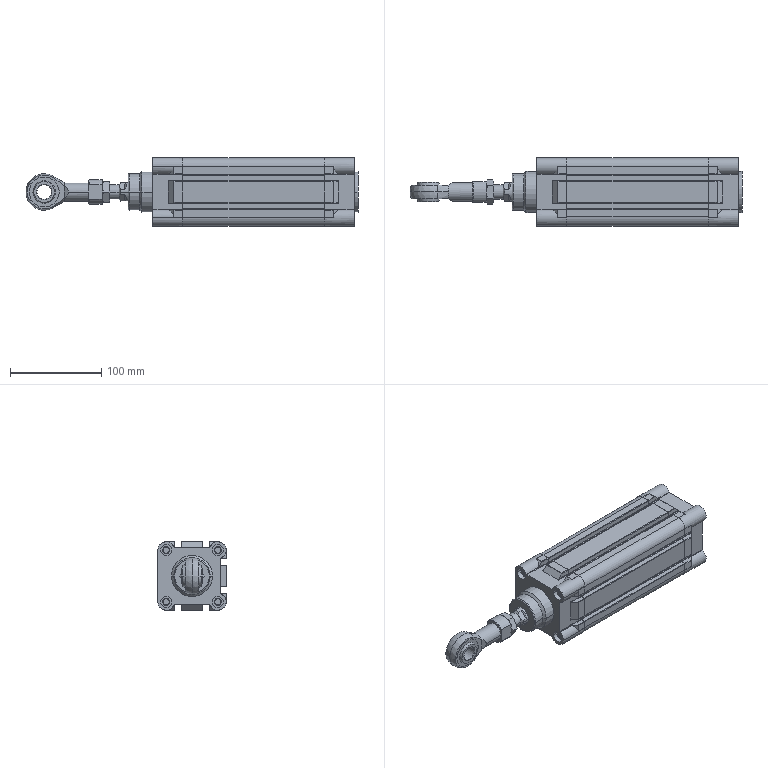Part | SolidWorks | 4 solids | 490 faces | box 364 x 75 x 75 mm | volume 905739 mm3 | cylinder 210 | plane 207 | cone 65 | spline 4 | torus 2 | sphere 2 | commonest cylinder face diameters 1 x102 20 x22 6.647 x16 12.4 x16 18.5 x10 5 x4